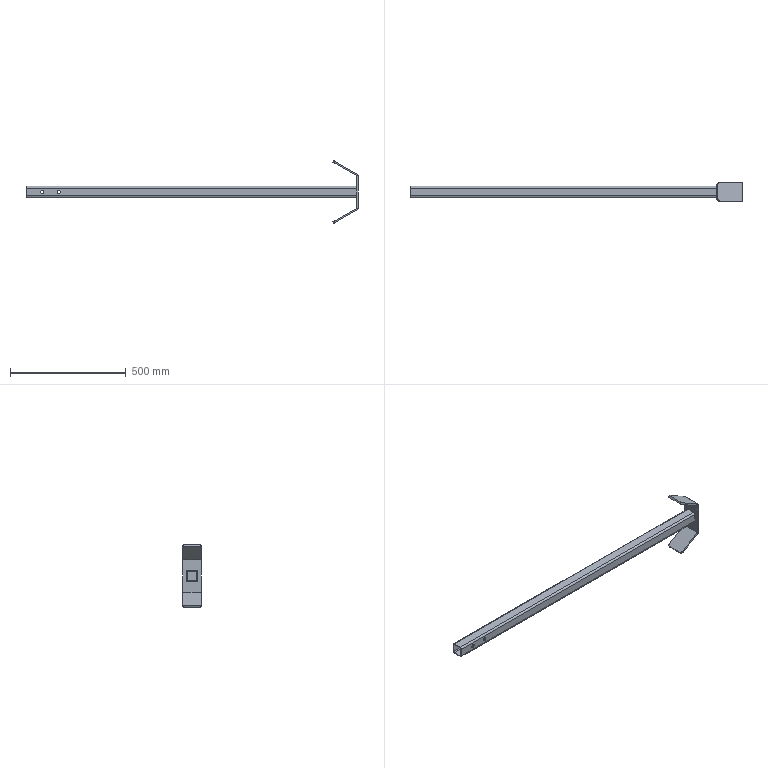Part | SolidWorks | features 3DProfileFeature 1, EdgeFlange 1, Fillet 1, FlatPattern 1, HoleWzd 1, SMBaseFlange 1, SheetMetal 1, WeldMemberFeat 1, WeldmentFeature 1 | 2 solids | 52 faces | box 1433 x 80 x 270.762 mm | volume 1230459 mm3 | plane 28 | cylinder 24 | commonest cylinder face diameters 14 x8 8 x4 16 x4 20 x4 1.473 x2 17.473 x2
STEP:
#1=CARTESIAN_POINT('',(70.,21.,7.));
#2=VERTEX_POINT('',#1);
#3=CARTESIAN_POINT('',(70.,21.,-7.));
#4=VERTEX_POINT('',#3);
#5=CARTESIAN_POINT('',(70.,21.,0.));
#6=DIRECTION('',(0.,-1.,0.));
#7=DIRECTION('',(0.,0.,-1.));
#8=AXIS2_PLACEMENT_3D('',#5,#6,#7);
#9=CIRCLE('',#8,7.);
#10=EDGE_CURVE('',#2,#4,#9,.T.);
#11=ORIENTED_EDGE('',*,*,#10,.T.);
#12=CARTESIAN_POINT('',(70.,25.,-7.));
#13=VERTEX_POINT('',#12);
#14=CARTESIAN_POINT('',(70.,25.,-7.));
#15=DIRECTION('',(0.,1.,0.));
#16=VECTOR('',#15,1000.);
#17=LINE('',#14,#16);
#18=EDGE_CURVE('',#4,#13,#17,.T.);
#19=ORIENTED_EDGE('',*,*,#18,.T.);
#20=CARTESIAN_POINT('',(70.,25.,7.));
#21=VERTEX_POINT('',#20);
#22=CARTESIAN_POINT('',(70.,25.,0.));
#23=DIRECTION('',(0.,1.,0.));
#24=DIRECTION('',(0.,0.,1.));
#25=AXIS2_PLACEMENT_3D('',#22,#23,#24);
#26=CIRCLE('',#25,7.);
#27=EDGE_CURVE('',#13,#21,#26,.T.);
#28=ORIENTED_EDGE('',*,*,#27,.T.);
#29=CARTESIAN_POINT('',(70.,25.,7.));
#30=DIRECTION('',(0.,1.,0.));
#31=VECTOR('',#30,1000.);
#32=LINE('',#29,#31);
#33=EDGE_CURVE('',#2,#21,#32,.T.);
#34=ORIENTED_EDGE('',*,*,#33,.F.);
#35=EDGE_LOOP('',(#11,#19,#28,#34));
#36=FACE_OUTER_BOUND('',#35,.T.);
#37=CARTESIAN_POINT('',(70.,25.,0.));
#38=DIRECTION('',(0.,1.,0.));
#39=DIRECTION('',(0.,0.,1.));
#40=AXIS2_PLACEMENT_3D('',#37,#38,#39);
#41=CYLINDRICAL_SURFACE('',#40,7.);
#42=ADVANCED_FACE('',(#36),#41,.F.);
#43=CARTESIAN_POINT('',(70.,-25.,7.));
#44=VERTEX_POINT('',#43);
#45=CARTESIAN_POINT('',(70.,-25.,-7.));
#46=VERTEX_POINT('',#45);
#47=CARTESIAN_POINT('',(70.,-25.,0.));
#48=DIRECTION('',(0.,-1.,0.));
#49=DIRECTION('',(0.,0.,1.));
#50=AXIS2_PLACEMENT_3D('',#47,#48,#49);
#51=CIRCLE('',#50,7.);
#52=EDGE_CURVE('',#44,#46,#51,.T.);
#53=ORIENTED_EDGE('',*,*,#52,.T.);
#54=CARTESIAN_POINT('',(70.,-21.,-7.));
#55=VERTEX_POINT('',#54);
#56=CARTESIAN_POINT('',(70.,25.,-7.));
#57=DIRECTION('',(0.,1.,0.));
#58=VECTOR('',#57,1000.);
#59=LINE('',#56,#58);
#60=EDGE_CURVE('',#46,#55,#59,.T.);
#61=ORIENTED_EDGE('',*,*,#60,.T.);
#62=CARTESIAN_POINT('',(70.,-21.,7.));
#63=VERTEX_POINT('',#62);
#64=CARTESIAN_POINT('',(70.,-21.,0.));
#65=DIRECTION('',(0.,1.,0.));
#66=DIRECTION('',(0.,0.,1.));
#67=AXIS2_PLACEMENT_3D('',#64,#65,#66);
#68=CIRCLE('',#67,7.);
#69=EDGE_CURVE('',#55,#63,#68,.T.);
#70=ORIENTED_EDGE('',*,*,#69,.T.);
#71=CARTESIAN_POINT('',(70.,25.,7.));
#72=DIRECTION('',(0.,1.,0.));
#73=VECTOR('',#72,1000.);
#74=LINE('',#71,#73);
#75=EDGE_CURVE('',#44,#63,#74,.T.);
#76=ORIENTED_EDGE('',*,*,#75,.F.);
#77=EDGE_LOOP('',(#53,#61,#70,#76));
#78=FACE_OUTER_BOUND('',#77,.T.);
#79=CARTESIAN_POINT('',(70.,25.,0.));
#80=DIRECTION('',(0.,1.,0.));
#81=DIRECTION('',(0.,0.,1.));
#82=AXIS2_PLACEMENT_3D('',#79,#80,#81);
#83=CYLINDRICAL_SURFACE('',#82,7.);
#84=ADVANCED_FACE('',(#78),#83,.F.);
#85=CARTESIAN_POINT('',(141.,21.,7.));
#86=VERTEX_POINT('',#85);
#87=CARTESIAN_POINT('',(141.,21.,-7.));
#88=VERTEX_POINT('',#87);
#89=CARTESIAN_POINT('',(141.,21.,0.));
#90=DIRECTION('',(0.,-1.,0.));
#91=DIRECTION('',(0.,0.,-1.));
#92=AXIS2_PLACEMENT_3D('',#89,#90,#91);
#93=CIRCLE('',#92,7.);
#94=EDGE_CURVE('',#86,#88,#93,.T.);
#95=ORIENTED_EDGE('',*,*,#94,.T.);
#96=CARTESIAN_POINT('',(141.,25.,-7.));
#97=VERTEX_POINT('',#96);
#98=CARTESIAN_POINT('',(141.,25.,-7.));
#99=DIRECTION('',(0.,1.,0.));
#100=VECTOR('',#99,1000.);
#101=LINE('',#98,#100);
#102=EDGE_CURVE('',#88,#97,#101,.T.);
#103=ORIENTED_EDGE('',*,*,#102,.T.);
#104=CARTESIAN_POINT('',(141.,25.,7.));
#105=VERTEX_POINT('',#104);
#106=CARTESIAN_POINT('',(141.,25.,0.));
#107=DIRECTION('',(0.,1.,0.));
#108=DIRECTION('',(0.,0.,1.));
#109=AXIS2_PLACEMENT_3D('',#106,#107,#108);
#110=CIRCLE('',#109,7.);
#111=EDGE_CURVE('',#97,#105,#110,.T.);
#112=ORIENTED_EDGE('',*,*,#111,.T.);
#113=CARTESIAN_POINT('',(141.,25.,7.));
#114=DIRECTION('',(0.,1.,0.));
#115=VECTOR('',#114,1000.);
#116=LINE('',#113,#115);
#117=EDGE_CURVE('',#86,#105,#116,.T.);
#118=ORIENTED_EDGE('',*,*,#117,.F.);
#119=EDGE_LOOP('',(#95,#103,#112,#118));
#120=FACE_OUTER_BOUND('',#119,.T.);
#121=CARTESIAN_POINT('',(141.,25.,0.));
#122=DIRECTION('',(0.,1.,0.));
#123=DIRECTION('',(0.,0.,1.));
#124=AXIS2_PLACEMENT_3D('',#121,#122,#123);
#125=CYLINDRICAL_SURFACE('',#124,7.);
#126=ADVANCED_FACE('',(#120),#125,.F.);
#127=CARTESIAN_POINT('',(141.,-25.,7.));
#128=VERTEX_POINT('',#127);
#129=CARTESIAN_POINT('',(141.,-25.,-7.));
#130=VERTEX_POINT('',#129);
#131=CARTESIAN_POINT('',(141.,-25.,0.));
#132=DIRECTION('',(0.,-1.,0.));
#133=DIRECTION('',(0.,0.,1.));
#134=AXIS2_PLACEMENT_3D('',#131,#132,#133);
#135=CIRCLE('',#134,7.);
#136=EDGE_CURVE('',#128,#130,#135,.T.);
#137=ORIENTED_EDGE('',*,*,#136,.T.);
#138=CARTESIAN_POINT('',(141.,-21.,-7.));
#139=VERTEX_POINT('',#138);
#140=CARTESIAN_POINT('',(141.,25.,-7.));
#141=DIRECTION('',(0.,1.,0.));
#142=VECTOR('',#141,1000.);
#143=LINE('',#140,#142);
#144=EDGE_CURVE('',#130,#139,#143,.T.);
#145=ORIENTED_EDGE('',*,*,#144,.T.);
#146=CARTESIAN_POINT('',(141.,-21.,7.));
#147=VERTEX_POINT('',#146);
#148=CARTESIAN_POINT('',(141.,-21.,0.));
#149=DIRECTION('',(0.,1.,0.));
#150=DIRECTION('',(0.,0.,1.));
#151=AXIS2_PLACEMENT_3D('',#148,#149,#150);
#152=CIRCLE('',#151,7.);
#153=EDGE_CURVE('',#139,#147,#152,.T.);
#154=ORIENTED_EDGE('',*,*,#153,.T.);
#155=CARTESIAN_POINT('',(141.,25.,7.));
#156=DIRECTION('',(0.,1.,0.));
#157=VECTOR('',#156,1000.);
#158=LINE('',#155,#157);
#159=EDGE_CURVE('',#128,#147,#158,.T.);
#160=ORIENTED_EDGE('',*,*,#159,.F.);
#161=EDGE_LOOP('',(#137,#145,#154,#160));
#162=FACE_OUTER_BOUND('',#161,.T.);
#163=CARTESIAN_POINT('',(141.,25.,0.));
#164=DIRECTION('',(0.,1.,0.));
#165=DIRECTION('',(0.,0.,1.));
#166=AXIS2_PLACEMENT_3D('',#163,#164,#165);
#167=CYLINDRICAL_SURFACE('',#166,7.);
#168=ADVANCED_FACE('',(#162),#167,.F.);
#169=CARTESIAN_POINT('',(0.,17.,-25.));
#170=VERTEX_POINT('',#169);
#171=CARTESIAN_POINT('',(0.,25.,-17.));
#172=VERTEX_POINT('',#171);
#173=CARTESIAN_POINT('',(0.,17.,-17.));
#174=DIRECTION('',(1.,0.,0.));
#175=DIRECTION('',(0.,0.,-1.));
#176=AXIS2_PLACEMENT_3D('',#173,#174,#175);
#177=CIRCLE('',#176,8.);
#178=EDGE_CURVE('',#170,#172,#177,.T.);
#179=ORIENTED_EDGE('',*,*,#178,.T.);
#180=CARTESIAN_POINT('',(1425.,25.,-17.));
#181=VERTEX_POINT('',#180);
#182=CARTESIAN_POINT('',(1425.,25.,-17.));
#183=DIRECTION('',(-1.,0.,0.));
#184=VECTOR('',#183,1000.);
#185=LINE('',#182,#184);
#186=EDGE_CURVE('',#181,#172,#185,.T.);
#187=ORIENTED_EDGE('',*,*,#186,.F.);
#188=CARTESIAN_POINT('',(1425.,17.,-25.));
#189=VERTEX_POINT('',#188);
#190=CARTESIAN_POINT('',(1425.,17.,-17.));
#191=DIRECTION('',(1.,0.,0.));
#192=DIRECTION('',(0.,0.,-1.));
#193=AXIS2_PLACEMENT_3D('',#190,#191,#192);
#194=CIRCLE('',#193,8.);
#195=EDGE_CURVE('',#189,#181,#194,.T.);
#196=ORIENTED_EDGE('',*,*,#195,.F.);
#197=CARTESIAN_POINT('',(1425.,17.,-25.));
#198=DIRECTION('',(-1.,0.,0.));
#199=VECTOR('',#198,1000.);
#200=LINE('',#197,#199);
#201=EDGE_CURVE('',#189,#170,#200,.T.);
#202=ORIENTED_EDGE('',*,*,#201,.T.);
#203=EDGE_LOOP('',(#179,#187,#196,#202));
#204=FACE_OUTER_BOUND('',#203,.T.);
#205=CARTESIAN_POINT('',(1425.,17.,-17.));
#206=DIRECTION('',(-1.,0.,0.));
#207=DIRECTION('',(0.,0.,1.));
#208=AXIS2_PLACEMENT_3D('',#205,#206,#207);
#209=CYLINDRICAL_SURFACE('',#208,8.);
#210=ADVANCED_FACE('',(#204),#209,.T.);
#211=CARTESIAN_POINT('',(70.,25.,0.));
#212=DIRECTION('',(0.,1.,0.));
#213=DIRECTION('',(0.,0.,1.));
#214=AXIS2_PLACEMENT_3D('',#211,#212,#213);
#215=CIRCLE('',#214,7.);
#216=EDGE_CURVE('',#21,#13,#215,.T.);
#217=ORIENTED_EDGE('',*,*,#216,.F.);
#218=ORIENTED_EDGE('',*,*,#27,.F.);
#219=EDGE_LOOP('',(#217,#218));
#220=FACE_BOUND('',#219,.T.);
#221=CARTESIAN_POINT('',(141.,25.,0.));
#222=DIRECTION('',(0.,1.,0.));
#223=DIRECTION('',(0.,0.,1.));
#224=AXIS2_PLACEMENT_3D('',#221,#222,#223);
#225=CIRCLE('',#224,7.);
#226=EDGE_CURVE('',#105,#97,#225,.T.);
#227=ORIENTED_EDGE('',*,*,#226,.F.);
#228=ORIENTED_EDGE('',*,*,#111,.F.);
#229=EDGE_LOOP('',(#227,#228));
#230=FACE_BOUND('',#229,.T.);
#231=CARTESIAN_POINT('',(0.,25.,17.));
#232=VERTEX_POINT('',#231);
#233=CARTESIAN_POINT('',(0.,25.,-17.));
#234=DIRECTION('',(0.,0.,1.));
#235=VECTOR('',#234,1000.);
#236=LINE('',#233,#235);
#237=EDGE_CURVE('',#172,#232,#236,.T.);
#238=ORIENTED_EDGE('',*,*,#237,.T.);
#239=CARTESIAN_POINT('',(1425.,25.,17.));
#240=VERTEX_POINT('',#239);
#241=CARTESIAN_POINT('',(1425.,25.,17.));
#242=DIRECTION('',(-1.,0.,0.));
#243=VECTOR('',#242,1000.);
#244=LINE('',#241,#243);
#245=EDGE_CURVE('',#240,#232,#244,.T.);
#246=ORIENTED_EDGE('',*,*,#245,.F.);
#247=CARTESIAN_POINT('',(1425.,25.,-17.));
#248=DIRECTION('',(0.,0.,1.));
#249=VECTOR('',#248,1000.);
#250=LINE('',#247,#249);
#251=EDGE_CURVE('',#181,#240,#250,.T.);
#252=ORIENTED_EDGE('',*,*,#251,.F.);
#253=ORIENTED_EDGE('',*,*,#186,.T.);
#254=EDGE_LOOP('',(#238,#246,#252,#253));
#255=FACE_OUTER_BOUND('',#254,.T.);
#256=CARTESIAN_POINT('',(1425.,25.,-17.));
#257=DIRECTION('',(0.,-1.,0.));
#258=DIRECTION('',(0.,0.,-1.));
#259=AXIS2_PLACEMENT_3D('',#256,#257,#258);
#260=PLANE('',#259);
#261=ADVANCED_FACE('',(#220,#230,#255),#260,.F.);
#262=CARTESIAN_POINT('',(0.,17.,25.));
#263=VERTEX_POINT('',#262);
#264=CARTESIAN_POINT('',(0.,17.,17.));
#265=DIRECTION('',(1.,0.,0.));
#266=DIRECTION('',(0.,0.,-1.));
#267=AXIS2_PLACEMENT_3D('',#264,#265,#266);
#268=CIRCLE('',#267,8.);
#269=EDGE_CURVE('',#232,#263,#268,.T.);
#270=ORIENTED_EDGE('',*,*,#269,.T.);
#271=CARTESIAN_POINT('',(1425.,17.,25.));
#272=VERTEX_POINT('',#271);
#273=CARTESIAN_POINT('',(1425.,17.,25.));
#274=DIRECTION('',(-1.,0.,0.));
#275=VECTOR('',#274,1000.);
#276=LINE('',#273,#275);
#277=EDGE_CURVE('',#272,#263,#276,.T.);
#278=ORIENTED_EDGE('',*,*,#277,.F.);
#279=CARTESIAN_POINT('',(1425.,17.,17.));
#280=DIRECTION('',(1.,0.,0.));
#281=DIRECTION('',(0.,0.,-1.));
#282=AXIS2_PLACEMENT_3D('',#279,#280,#281);
#283=CIRCLE('',#282,8.);
#284=EDGE_CURVE('',#240,#272,#283,.T.);
#285=ORIENTED_EDGE('',*,*,#284,.F.);
#286=ORIENTED_EDGE('',*,*,#245,.T.);
#287=EDGE_LOOP('',(#270,#278,#285,#286));
#288=FACE_OUTER_BOUND('',#287,.T.);
#289=CARTESIAN_POINT('',(1425.,17.,17.));
#290=DIRECTION('',(-1.,0.,0.));
#291=DIRECTION('',(0.,0.,1.));
#292=AXIS2_PLACEMENT_3D('',#289,#290,#291);
#293=CYLINDRICAL_SURFACE('',#292,8.);
#294=ADVANCED_FACE('',(#288),#293,.T.);
#295=CARTESIAN_POINT('',(0.,-17.,25.));
#296=VERTEX_POINT('',#295);
#297=CARTESIAN_POINT('',(0.,-17.,25.));
#298=DIRECTION('',(0.,-1.,0.));
#299=VECTOR('',#298,1000.);
#300=LINE('',#297,#299);
#301=EDGE_CURVE('',#263,#296,#300,.T.);
#302=ORIENTED_EDGE('',*,*,#301,.T.);
#303=CARTESIAN_POINT('',(1425.,-17.,25.));
#304=VERTEX_POINT('',#303);
#305=CARTESIAN_POINT('',(1425.,-17.,25.));
#306=DIRECTION('',(-1.,0.,0.));
#307=VECTOR('',#306,1000.);
#308=LINE('',#305,#307);
#309=EDGE_CURVE('',#304,#296,#308,.T.);
#310=ORIENTED_EDGE('',*,*,#309,.F.);
#311=CARTESIAN_POINT('',(1425.,-17.,25.));
#312=DIRECTION('',(0.,-1.,0.));
#313=VECTOR('',#312,1000.);
#314=LINE('',#311,#313);
#315=EDGE_CURVE('',#272,#304,#314,.T.);
#316=ORIENTED_EDGE('',*,*,#315,.F.);
#317=ORIENTED_EDGE('',*,*,#277,.T.);
#318=EDGE_LOOP('',(#302,#310,#316,#317));
#319=FACE_OUTER_BOUND('',#318,.T.);
#320=CARTESIAN_POINT('',(1425.,-17.,25.));
#321=DIRECTION('',(0.,0.,-1.));
#322=DIRECTION('',(-1.,0.,0.));
#323=AXIS2_PLACEMENT_3D('',#320,#321,#322);
#324=PLANE('',#323);
#325=ADVANCED_FACE('',(#319),#324,.F.);
#326=CARTESIAN_POINT('',(0.,-25.,17.));
#327=VERTEX_POINT('',#326);
#328=CARTESIAN_POINT('',(0.,-17.,17.));
#329=DIRECTION('',(1.,0.,0.));
#330=DIRECTION('',(0.,0.,-1.));
#331=AXIS2_PLACEMENT_3D('',#328,#329,#330);
#332=CIRCLE('',#331,8.);
#333=EDGE_CURVE('',#296,#327,#332,.T.);
#334=ORIENTED_EDGE('',*,*,#333,.T.);
#335=CARTESIAN_POINT('',(1425.,-25.,17.));
#336=VERTEX_POINT('',#335);
#337=CARTESIAN_POINT('',(1425.,-25.,17.));
#338=DIRECTION('',(-1.,0.,0.));
#339=VECTOR('',#338,1000.);
#340=LINE('',#337,#339);
#341=EDGE_CURVE('',#336,#327,#340,.T.);
#342=ORIENTED_EDGE('',*,*,#341,.F.);
#343=CARTESIAN_POINT('',(1425.,-17.,17.));
#344=DIRECTION('',(1.,0.,0.));
#345=DIRECTION('',(0.,0.,-1.));
#346=AXIS2_PLACEMENT_3D('',#343,#344,#345);
#347=CIRCLE('',#346,8.);
#348=EDGE_CURVE('',#304,#336,#347,.T.);
#349=ORIENTED_EDGE('',*,*,#348,.F.);
#350=ORIENTED_EDGE('',*,*,#309,.T.);
#351=EDGE_LOOP('',(#334,#342,#349,#350));
#352=FACE_OUTER_BOUND('',#351,.T.);
#353=CARTESIAN_POINT('',(1425.,-17.,17.));
#354=DIRECTION('',(-1.,0.,0.));
#355=DIRECTION('',(0.,0.,1.));
#356=AXIS2_PLACEMENT_3D('',#353,#354,#355);
#357=CYLINDRICAL_SURFACE('',#356,8.);
#358=ADVANCED_FACE('',(#352),#357,.T.);
#359=ORIENTED_EDGE('',*,*,#52,.F.);
#360=CARTESIAN_POINT('',(70.,-25.,0.));
#361=DIRECTION('',(0.,-1.,0.));
#362=DIRECTION('',(0.,0.,1.));
#363=AXIS2_PLACEMENT_3D('',#360,#361,#362);
#364=CIRCLE('',#363,7.);
#365=EDGE_CURVE('',#46,#44,#364,.T.);
#366=ORIENTED_EDGE('',*,*,#365,.F.);
#367=EDGE_LOOP('',(#359,#366));
#368=FACE_BOUND('',#367,.T.);
#369=ORIENTED_EDGE('',*,*,#136,.F.);
#370=CARTESIAN_POINT('',(141.,-25.,0.));
#371=DIRECTION('',(0.,-1.,0.));
#372=DIRECTION('',(0.,0.,1.));
#373=AXIS2_PLACEMENT_3D('',#370,#371,#372);
#374=CIRCLE('',#373,7.);
#375=EDGE_CURVE('',#130,#128,#374,.T.);
#376=ORIENTED_EDGE('',*,*,#375,.F.);
#377=EDGE_LOOP('',(#369,#376));
#378=FACE_BOUND('',#377,.T.);
#379=CARTESIAN_POINT('',(0.,-25.,-17.));
#380=VERTEX_POINT('',#379);
#381=CARTESIAN_POINT('',(0.,-25.,17.));
#382=DIRECTION('',(0.,0.,-1.));
#383=VECTOR('',#382,1000.);
#384=LINE('',#381,#383);
#385=EDGE_CURVE('',#327,#380,#384,.T.);
#386=ORIENTED_EDGE('',*,*,#385,.T.);
#387=CARTESIAN_POINT('',(1425.,-25.,-17.));
#388=VERTEX_POINT('',#387);
#389=CARTESIAN_POINT('',(1425.,-25.,-17.));
#390=DIRECTION('',(-1.,0.,0.));
#391=VECTOR('',#390,1000.);
#392=LINE('',#389,#391);
#393=EDGE_CURVE('',#388,#380,#392,.T.);
#394=ORIENTED_EDGE('',*,*,#393,.F.);
#395=CARTESIAN_POINT('',(1425.,-25.,17.));
#396=DIRECTION('',(0.,0.,-1.));
#397=VECTOR('',#396,1000.);
#398=LINE('',#395,#397);
#399=EDGE_CURVE('',#336,#388,#398,.T.);
#400=ORIENTED_EDGE('',*,*,#399,.F.);
#401=ORIENTED_EDGE('',*,*,#341,.T.);
#402=EDGE_LOOP('',(#386,#394,#400,#401));
#403=FACE_OUTER_BOUND('',#402,.T.);
#404=CARTESIAN_POINT('',(1425.,-25.,17.));
#405=DIRECTION('',(0.,1.,0.));
#406=DIRECTION('',(0.,0.,1.));
#407=AXIS2_PLACEMENT_3D('',#404,#405,#406);
#408=PLANE('',#407);
#409=ADVANCED_FACE('',(#368,#378,#403),#408,.F.);
#410=CARTESIAN_POINT('',(0.,-17.,-25.));
#411=VERTEX_POINT('',#410);
#412=CARTESIAN_POINT('',(0.,-17.,-17.));
#413=DIRECTION('',(1.,0.,0.));
#414=DIRECTION('',(0.,0.,-1.));
#415=AXIS2_PLACEMENT_3D('',#412,#413,#414);
#416=CIRCLE('',#415,8.);
#417=EDGE_CURVE('',#380,#411,#416,.T.);
#418=ORIENTED_EDGE('',*,*,#417,.T.);
#419=CARTESIAN_POINT('',(1425.,-17.,-25.));
#420=VERTEX_POINT('',#419);
#421=CARTESIAN_POINT('',(1425.,-17.,-25.));
#422=DIRECTION('',(-1.,0.,0.));
#423=VECTOR('',#422,1000.);
#424=LINE('',#421,#423);
#425=EDGE_CURVE('',#420,#411,#424,.T.);
#426=ORIENTED_EDGE('',*,*,#425,.F.);
#427=CARTESIAN_POINT('',(1425.,-17.,-17.));
#428=DIRECTION('',(1.,0.,0.));
#429=DIRECTION('',(0.,0.,-1.));
#430=AXIS2_PLACEMENT_3D('',#427,#428,#429);
#431=CIRCLE('',#430,8.);
#432=EDGE_CURVE('',#388,#420,#431,.T.);
#433=ORIENTED_EDGE('',*,*,#432,.F.);
#434=ORIENTED_EDGE('',*,*,#393,.T.);
#435=EDGE_LOOP('',(#418,#426,#433,#434));
#436=FACE_OUTER_BOUND('',#435,.T.);
#437=CARTESIAN_POINT('',(1425.,-17.,-17.));
#438=DIRECTION('',(-1.,0.,0.));
#439=DIRECTION('',(0.,0.,1.));
#440=AXIS2_PLACEMENT_3D('',#437,#438,#439);
#441=CYLINDRICAL_SURFACE('',#440,8.);
#442=ADVANCED_FACE('',(#436),#441,.T.);
#443=CARTESIAN_POINT('',(0.,21.,17.));
#444=VERTEX_POINT('',#443);
#445=CARTESIAN_POINT('',(0.,17.,21.));
#446=VERTEX_POINT('',#445);
#447=CARTESIAN_POINT('',(0.,17.,17.));
#448=DIRECTION('',(1.,0.,0.));
#449=DIRECTION('',(0.,0.,-1.));
#450=AXIS2_PLACEMENT_3D('',#447,#448,#449);
#451=CIRCLE('',#450,4.);
#452=EDGE_CURVE('',#444,#446,#451,.T.);
#453=ORIENTED_EDGE('',*,*,#452,.F.);
#454=CARTESIAN_POINT('',(1425.,21.,17.));
#455=VERTEX_POINT('',#454);
#456=CARTESIAN_POINT('',(1425.,21.,17.));
#457=DIRECTION('',(-1.,0.,0.));
#458=VECTOR('',#457,1000.);
#459=LINE('',#456,#458);
#460=EDGE_CURVE('',#455,#444,#459,.T.);
#461=ORIENTED_EDGE('',*,*,#460,.F.);
#462=CARTESIAN_POINT('',(1425.,17.,21.));
#463=VERTEX_POINT('',#462);
#464=CARTESIAN_POINT('',(1425.,17.,17.));
#465=DIRECTION('',(1.,0.,0.));
#466=DIRECTION('',(0.,0.,-1.));
#467=AXIS2_PLACEMENT_3D('',#464,#465,#466);
#468=CIRCLE('',#467,4.);
#469=EDGE_CURVE('',#455,#463,#468,.T.);
#470=ORIENTED_EDGE('',*,*,#469,.T.);
#471=CARTESIAN_POINT('',(1425.,17.,21.));
#472=DIRECTION('',(-1.,0.,0.));
#473=VECTOR('',#472,1000.);
#474=LINE('',#471,#473);
#475=EDGE_CURVE('',#463,#446,#474,.T.);
#476=ORIENTED_EDGE('',*,*,#475,.T.);
#477=EDGE_LOOP('',(#453,#461,#470,#476));
#478=FACE_OUTER_BOUND('',#477,.T.);
#479=CARTESIAN_POINT('',(1425.,17.,17.));
#480=DIRECTION('',(-1.,0.,0.));
#481=DIRECTION('',(0.,0.,1.));
#482=AXIS2_PLACEMENT_3D('',#479,#480,#481);
#483=CYLINDRICAL_SURFACE('',#482,4.);
#484=ADVANCED_FACE('',(#478),#483,.F.);
#485=ORIENTED_EDGE('',*,*,#10,.F.);
#486=CARTESIAN_POINT('',(70.,21.,0.));
#487=DIRECTION('',(0.,-1.,0.));
#488=DIRECTION('',(0.,0.,-1.));
#489=AXIS2_PLACEMENT_3D('',#486,#487,#488);
#490=CIRCLE('',#489,7.);
#491=EDGE_CURVE('',#4,#2,#490,.T.);
#492=ORIENTED_EDGE('',*,*,#491,.F.);
#493=EDGE_LOOP('',(#485,#492));
#494=FACE_BOUND('',#493,.T.);
#495=ORIENTED_EDGE('',*,*,#94,.F.);
#496=CARTESIAN_POINT('',(141.,21.,0.));
#497=DIRECTION('',(0.,-1.,0.));
#498=DIRECTION('',(0.,0.,-1.));
#499=AXIS2_PLACEMENT_3D('',#496,#497,#498);
#500=CIRCLE('',#499,7.);
#501=EDGE_CURVE('',#88,#86,#500,.T.);
#502=ORIENTED_EDGE('',*,*,#501,.F.);
#503=EDGE_LOOP('',(#495,#502));
#504=FACE_BOUND('',#503,.T.);
#505=CARTESIAN_POINT('',(0.,21.,-17.));
#506=VERTEX_POINT('',#505);
#507=CARTESIAN_POINT('',(0.,21.,-17.));
#508=DIRECTION('',(0.,0.,1.));
#509=VECTOR('',#508,1000.);
#510=LINE('',#507,#509);
#511=EDGE_CURVE('',#506,#444,#510,.T.);
#512=ORIENTED_EDGE('',*,*,#511,.F.);
#513=CARTESIAN_POINT('',(1425.,21.,-17.));
#514=VERTEX_POINT('',#513);
#515=CARTESIAN_POINT('',(1425.,21.,-17.));
#516=DIRECTION('',(-1.,0.,0.));
#517=VECTOR('',#516,1000.);
#518=LINE('',#515,#517);
#519=EDGE_CURVE('',#514,#506,#518,.T.);
#520=ORIENTED_EDGE('',*,*,#519,.F.);
#521=CARTESIAN_POINT('',(1425.,21.,-17.));
#522=DIRECTION('',(0.,0.,1.));
#523=VECTOR('',#522,1000.);
#524=LINE('',#521,#523);
#525=EDGE_CURVE('',#514,#455,#524,.T.);
#526=ORIENTED_EDGE('',*,*,#525,.T.);
#527=ORIENTED_EDGE('',*,*,#460,.T.);
#528=EDGE_LOOP('',(#512,#520,#526,#527));
#529=FACE_OUTER_BOUND('',#528,.T.);
#530=CARTESIAN_POINT('',(1425.,21.,-17.));
#531=DIRECTION('',(0.,-1.,0.));
#532=DIRECTION('',(0.,0.,-1.));
#533=AXIS2_PLACEMENT_3D('',#530,#531,#532);
#534=PLANE('',#533);
#535=ADVANCED_FACE('',(#494,#504,#529),#534,.T.);
#536=CARTESIAN_POINT('',(0.,17.,-21.));
#537=VERTEX_POINT('',#536);
#538=CARTESIAN_POINT('',(0.,17.,-17.));
#539=DIRECTION('',(1.,0.,0.));
#540=DIRECTION('',(0.,0.,-1.));
#541=AXIS2_PLACEMENT_3D('',#538,#539,#540);
#542=CIRCLE('',#541,4.);
#543=EDGE_CURVE('',#537,#506,#542,.T.);
#544=ORIENTED_EDGE('',*,*,#543,.F.);
#545=CARTESIAN_POINT('',(1425.,17.,-21.));
#546=VERTEX_POINT('',#545);
#547=CARTESIAN_POINT('',(1425.,17.,-21.));
#548=DIRECTION('',(-1.,0.,0.));
#549=VECTOR('',#548,1000.);
#550=LINE('',#547,#549);
#551=EDGE_CURVE('',#546,#537,#550,.T.);
#552=ORIENTED_EDGE('',*,*,#551,.F.);
#553=CARTESIAN_POINT('',(1425.,17.,-17.));
#554=DIRECTION('',(1.,0.,0.));
#555=DIRECTION('',(0.,0.,-1.));
#556=AXIS2_PLACEMENT_3D('',#553,#554,#555);
#557=CIRCLE('',#556,4.);
#558=EDGE_CURVE('',#546,#514,#557,.T.);
#559=ORIENTED_EDGE('',*,*,#558,.T.);
#560=ORIENTED_EDGE('',*,*,#519,.T.);
#561=EDGE_LOOP('',(#544,#552,#559,#560));
#562=FACE_OUTER_BOUND('',#561,.T.);
#563=CARTESIAN_POINT('',(1425.,17.,-17.));
#564=DIRECTION('',(-1.,0.,0.));
#565=DIRECTION('',(0.,0.,1.));
#566=AXIS2_PLACEMENT_3D('',#563,#564,#565);
#567=CYLINDRICAL_SURFACE('',#566,4.);
#568=ADVANCED_FACE('',(#562),#567,.F.);
#569=CARTESIAN_POINT('',(0.,-17.,-21.));
#570=VERTEX_POINT('',#569);
#571=CARTESIAN_POINT('',(0.,17.,-21.));
#572=DIRECTION('',(0.,1.,0.));
#573=VECTOR('',#572,1000.);
#574=LINE('',#571,#573);
#575=EDGE_CURVE('',#570,#537,#574,.T.);
#576=ORIENTED_EDGE('',*,*,#575,.F.);
#577=CARTESIAN_POINT('',(1425.,-17.,-21.));
#578=VERTEX_POINT('',#577);
#579=CARTESIAN_POINT('',(1425.,-17.,-21.));
#580=DIRECTION('',(-1.,0.,0.));
#581=VECTOR('',#580,1000.);
#582=LINE('',#579,#581);
#583=EDGE_CURVE('',#578,#570,#582,.T.);
#584=ORIENTED_EDGE('',*,*,#583,.F.);
#585=CARTESIAN_POINT('',(1425.,17.,-21.));
#586=DIRECTION('',(0.,1.,0.));
#587=VECTOR('',#586,1000.);
#588=LINE('',#585,#587);
#589=EDGE_CURVE('',#578,#546,#588,.T.);
#590=ORIENTED_EDGE('',*,*,#589,.T.);
#591=ORIENTED_EDGE('',*,*,#551,.T.);
#592=EDGE_LOOP('',(#576,#584,#590,#591));
#593=FACE_OUTER_BOUND('',#592,.T.);
#594=CARTESIAN_POINT('',(1425.,17.,-21.));
#595=DIRECTION('',(0.,0.,1.));
#596=DIRECTION('',(1.,0.,0.));
#597=AXIS2_PLACEMENT_3D('',#594,#595,#596);
#598=PLANE('',#597);
#599=ADVANCED_FACE('',(#593),#598,.T.);
#600=CARTESIAN_POINT('',(0.,-21.,-17.));
#601=VERTEX_POINT('',#600);
#602=CARTESIAN_POINT('',(0.,-17.,-17.));
#603=DIRECTION('',(1.,0.,0.));
#604=DIRECTION('',(0.,0.,-1.));
#605=AXIS2_PLACEMENT_3D('',#602,#603,#604);
#606=CIRCLE('',#605,4.);
#607=EDGE_CURVE('',#601,#570,#606,.T.);
#608=ORIENTED_EDGE('',*,*,#607,.F.);
#609=CARTESIAN_POINT('',(1425.,-21.,-17.));
#610=VERTEX_POINT('',#609);
#611=CARTESIAN_POINT('',(1425.,-21.,-17.));
#612=DIRECTION('',(-1.,0.,0.));
#613=VECTOR('',#612,1000.);
#614=LINE('',#611,#613);
#615=EDGE_CURVE('',#610,#601,#614,.T.);
#616=ORIENTED_EDGE('',*,*,#615,.F.);
#617=CARTESIAN_POINT('',(1425.,-17.,-17.));
#618=DIRECTION('',(1.,0.,0.));
#619=DIRECTION('',(0.,0.,-1.));
#620=AXIS2_PLACEMENT_3D('',#617,#618,#619);
#621=CIRCLE('',#620,4.);
#622=EDGE_CURVE('',#610,#578,#621,.T.);
#623=ORIENTED_EDGE('',*,*,#622,.T.);
#624=ORIENTED_EDGE('',*,*,#583,.T.);
#625=EDGE_LOOP('',(#608,#616,#623,#624));
#626=FACE_OUTER_BOUND('',#625,.T.);
#627=CARTESIAN_POINT('',(1425.,-17.,-17.));
#628=DIRECTION('',(-1.,0.,0.));
#629=DIRECTION('',(0.,0.,1.));
#630=AXIS2_PLACEMENT_3D('',#627,#628,#629);
#631=CYLINDRICAL_SURFACE('',#630,4.);
#632=ADVANCED_FACE('',(#626),#631,.F.);
#633=CARTESIAN_POINT('',(70.,-21.,0.));
#634=DIRECTION('',(0.,1.,0.));
#635=DIRECTION('',(0.,0.,1.));
#636=AXIS2_PLACEMENT_3D('',#633,#634,#635);
#637=CIRCLE('',#636,7.);
#638=EDGE_CURVE('',#63,#55,#637,.T.);
#639=ORIENTED_EDGE('',*,*,#638,.F.);
#640=ORIENTED_EDGE('',*,*,#69,.F.);
#641=EDGE_LOOP('',(#639,#640));
#642=FACE_BOUND('',#641,.T.);
#643=CARTESIAN_POINT('',(141.,-21.,0.));
#644=DIRECTION('',(0.,1.,0.));
#645=DIRECTION('',(0.,0.,1.));
#646=AXIS2_PLACEMENT_3D('',#643,#644,#645);
#647=CIRCLE('',#646,7.);
#648=EDGE_CURVE('',#147,#139,#647,.T.);
#649=ORIENTED_EDGE('',*,*,#648,.F.);
#650=ORIENTED_EDGE('',*,*,#153,.F.);
#651=EDGE_LOOP('',(#649,#650));
#652=FACE_BOUND('',#651,.T.);
#653=CARTESIAN_POINT('',(0.,-21.,17.));
#654=VERTEX_POINT('',#653);
#655=CARTESIAN_POINT('',(0.,-21.,17.));
#656=DIRECTION('',(0.,0.,-1.));
#657=VECTOR('',#656,1000.);
#658=LINE('',#655,#657);
#659=EDGE_CURVE('',#654,#601,#658,.T.);
#660=ORIENTED_EDGE('',*,*,#659,.F.);
#661=CARTESIAN_POINT('',(1425.,-21.,17.));
#662=VERTEX_POINT('',#661);
#663=CARTESIAN_POINT('',(1425.,-21.,17.));
#664=DIRECTION('',(-1.,0.,0.));
#665=VECTOR('',#664,1000.);
#666=LINE('',#663,#665);
#667=EDGE_CURVE('',#662,#654,#666,.T.);
#668=ORIENTED_EDGE('',*,*,#667,.F.);
#669=CARTESIAN_POINT('',(1425.,-21.,17.));
#670=DIRECTION('',(0.,0.,-1.));
#671=VECTOR('',#670,1000.);
#672=LINE('',#669,#671);
#673=EDGE_CURVE('',#662,#610,#672,.T.);
#674=ORIENTED_EDGE('',*,*,#673,.T.);
#675=ORIENTED_EDGE('',*,*,#615,.T.);
#676=EDGE_LOOP('',(#660,#668,#674,#675));
#677=FACE_OUTER_BOUND('',#676,.T.);
#678=CARTESIAN_POINT('',(1425.,-21.,17.));
#679=DIRECTION('',(0.,1.,0.));
#680=DIRECTION('',(0.,0.,1.));
#681=AXIS2_PLACEMENT_3D('',#678,#679,#680);
#682=PLANE('',#681);
#683=ADVANCED_FACE('',(#642,#652,#677),#682,.T.);
#684=CARTESIAN_POINT('',(0.,-17.,21.));
#685=VERTEX_POINT('',#684);
#686=CARTESIAN_POINT('',(0.,-17.,17.));
#687=DIRECTION('',(1.,0.,0.));
#688=DIRECTION('',(0.,0.,-1.));
#689=AXIS2_PLACEMENT_3D('',#686,#687,#688);
#690=CIRCLE('',#689,4.);
#691=EDGE_CURVE('',#685,#654,#690,.T.);
#692=ORIENTED_EDGE('',*,*,#691,.F.);
#693=CARTESIAN_POINT('',(1425.,-17.,21.));
#694=VERTEX_POINT('',#693);
#695=CARTESIAN_POINT('',(1425.,-17.,21.));
#696=DIRECTION('',(-1.,0.,0.));
#697=VECTOR('',#696,1000.);
#698=LINE('',#695,#697);
#699=EDGE_CURVE('',#694,#685,#698,.T.);
#700=ORIENTED_EDGE('',*,*,#699,.F.);
#701=CARTESIAN_POINT('',(1425.,-17.,17.));
#702=DIRECTION('',(1.,0.,0.));
#703=DIRECTION('',(0.,0.,-1.));
#704=AXIS2_PLACEMENT_3D('',#701,#702,#703);
#705=CIRCLE('',#704,4.);
#706=EDGE_CURVE('',#694,#662,#705,.T.);
#707=ORIENTED_EDGE('',*,*,#706,.T.);
#708=ORIENTED_EDGE('',*,*,#667,.T.);
#709=EDGE_LOOP('',(#692,#700,#707,#708));
#710=FACE_OUTER_BOUND('',#709,.T.);
#711=CARTESIAN_POINT('',(1425.,-17.,17.));
#712=DIRECTION('',(-1.,0.,0.));
#713=DIRECTION('',(0.,0.,1.));
#714=AXIS2_PLACEMENT_3D('',#711,#712,#713);
#715=CYLINDRICAL_SURFACE('',#714,4.);
#716=ADVANCED_FACE('',(#710),#715,.F.);
#717=CARTESIAN_POINT('',(0.,-17.,21.));
#718=DIRECTION('',(0.,-1.,0.));
#719=VECTOR('',#718,1000.);
#720=LINE('',#717,#719);
#721=EDGE_CURVE('',#446,#685,#720,.T.);
#722=ORIENTED_EDGE('',*,*,#721,.F.);
#723=ORIENTED_EDGE('',*,*,#475,.F.);
#724=CARTESIAN_POINT('',(1425.,-17.,21.));
#725=DIRECTION('',(0.,-1.,0.));
#726=VECTOR('',#725,1000.);
#727=LINE('',#724,#726);
#728=EDGE_CURVE('',#463,#694,#727,.T.);
#729=ORIENTED_EDGE('',*,*,#728,.T.);
#730=ORIENTED_EDGE('',*,*,#699,.T.);
#731=EDGE_LOOP('',(#722,#723,#729,#730));
#732=FACE_OUTER_BOUND('',#731,.T.);
#733=CARTESIAN_POINT('',(1425.,-17.,21.));
#734=DIRECTION('',(0.,0.,-1.));
#735=DIRECTION('',(-1.,0.,0.));
#736=AXIS2_PLACEMENT_3D('',#733,#734,#735);
#737=PLANE('',#736);
#738=ADVANCED_FACE('',(#732),#737,.T.);
#739=CARTESIAN_POINT('',(0.,17.,-25.));
#740=DIRECTION('',(0.,1.,0.));
#741=VECTOR('',#740,1000.);
#742=LINE('',#739,#741);
#743=EDGE_CURVE('',#411,#170,#742,.T.);
#744=ORIENTED_EDGE('',*,*,#743,.T.);
#745=ORIENTED_EDGE('',*,*,#201,.F.);
#746=CARTESIAN_POINT('',(1425.,17.,-25.));
#747=DIRECTION('',(0.,1.,0.));
#748=VECTOR('',#747,1000.);
#749=LINE('',#746,#748);
#750=EDGE_CURVE('',#420,#189,#749,.T.);
#751=ORIENTED_EDGE('',*,*,#750,.F.);
#752=ORIENTED_EDGE('',*,*,#425,.T.);
#753=EDGE_LOOP('',(#744,#745,#751,#752));
#754=FACE_OUTER_BOUND('',#753,.T.);
#755=CARTESIAN_POINT('',(1425.,17.,-25.));
#756=DIRECTION('',(0.,0.,1.));
#757=DIRECTION('',(1.,0.,0.));
#758=AXIS2_PLACEMENT_3D('',#755,#756,#757);
#759=PLANE('',#758);
#760=ADVANCED_FACE('',(#754),#759,.F.);
#761=ORIENTED_EDGE('',*,*,#469,.F.);
#762=ORIENTED_EDGE('',*,*,#525,.F.);
#763=ORIENTED_EDGE('',*,*,#558,.F.);
#764=ORIENTED_EDGE('',*,*,#589,.F.);
#765=ORIENTED_EDGE('',*,*,#622,.F.);
#766=ORIENTED_EDGE('',*,*,#673,.F.);
#767=ORIENTED_EDGE('',*,*,#706,.F.);
#768=ORIENTED_EDGE('',*,*,#728,.F.);
#769=EDGE_LOOP('',(#761,#762,#763,#764,#765,#766,#767,#768));
#770=FACE_BOUND('',#769,.T.);
#771=ORIENTED_EDGE('',*,*,#195,.T.);
#772=ORIENTED_EDGE('',*,*,#251,.T.);
#773=ORIENTED_EDGE('',*,*,#284,.T.);
#774=ORIENTED_EDGE('',*,*,#315,.T.);
#775=ORIENTED_EDGE('',*,*,#348,.T.);
#776=ORIENTED_EDGE('',*,*,#399,.T.);
#777=ORIENTED_EDGE('',*,*,#432,.T.);
#778=ORIENTED_EDGE('',*,*,#750,.T.);
#779=EDGE_LOOP('',(#771,#772,#773,#774,#775,#776,#777,#778));
#780=FACE_OUTER_BOUND('',#779,.T.);
#781=CARTESIAN_POINT('',(1425.,17.,-17.));
#782=DIRECTION('',(1.,0.,0.));
#783=DIRECTION('',(0.,0.,-1.));
#784=AXIS2_PLACEMENT_3D('',#781,#782,#783);
#785=PLANE('',#784);
#786=ADVANCED_FACE('',(#770,#780),#785,.T.);
#787=ORIENTED_EDGE('',*,*,#452,.T.);
#788=ORIENTED_EDGE('',*,*,#721,.T.);
#789=ORIENTED_EDGE('',*,*,#691,.T.);
#790=ORIENTED_EDGE('',*,*,#659,.T.);
#791=ORIENTED_EDGE('',*,*,#607,.T.);
#792=ORIENTED_EDGE('',*,*,#575,.T.);
#793=ORIENTED_EDGE('',*,*,#543,.T.);
#794=ORIENTED_EDGE('',*,*,#511,.T.);
#795=EDGE_LOOP('',(#787,#788,#789,#790,#791,#792,#793,#794));
#796=FACE_BOUND('',#795,.T.);
#797=ORIENTED_EDGE('',*,*,#178,.F.);
#798=ORIENTED_EDGE('',*,*,#743,.F.);
#799=ORIENTED_EDGE('',*,*,#417,.F.);
#800=ORIENTED_EDGE('',*,*,#385,.F.);
#801=ORIENTED_EDGE('',*,*,#333,.F.);
#802=ORIENTED_EDGE('',*,*,#301,.F.);
#803=ORIENTED_EDGE('',*,*,#269,.F.);
#804=ORIENTED_EDGE('',*,*,#237,.F.);
#805=EDGE_LOOP('',(#797,#798,#799,#800,#801,#802,#803,#804));
#806=FACE_OUTER_BOUND('',#805,.T.);
#807=CARTESIAN_POINT('',(0.,17.,-17.));
#808=DIRECTION('',(1.,0.,0.));
#809=DIRECTION('',(0.,0.,-1.));
#810=AXIS2_PLACEMENT_3D('',#807,#808,#809);
#811=PLANE('',#810);
#812=ADVANCED_FACE('',(#796,#806),#811,.F.);
#813=ORIENTED_EDGE('',*,*,#144,.F.);
#814=ORIENTED_EDGE('',*,*,#375,.T.);
#815=ORIENTED_EDGE('',*,*,#159,.T.);
#816=ORIENTED_EDGE('',*,*,#648,.T.);
#817=EDGE_LOOP('',(#813,#814,#815,#816));
#818=FACE_OUTER_BOUND('',#817,.T.);
#819=CARTESIAN_POINT('',(141.,25.,0.));
#820=DIRECTION('',(0.,1.,0.));
#821=DIRECTION('',(0.,0.,1.));
#822=AXIS2_PLACEMENT_3D('',#819,#820,#821);
#823=CYLINDRICAL_SURFACE('',#822,7.);
#824=ADVANCED_FACE('',(#818),#823,.F.);
#825=ORIENTED_EDGE('',*,*,#102,.F.);
#826=ORIENTED_EDGE('',*,*,#501,.T.);
#827=ORIENTED_EDGE('',*,*,#117,.T.);
#828=ORIENTED_EDGE('',*,*,#226,.T.);
#829=EDGE_LOOP('',(#825,#826,#827,#828));
#830=FACE_OUTER_BOUND('',#829,.T.);
#831=CARTESIAN_POINT('',(141.,25.,0.));
#832=DIRECTION('',(0.,1.,0.));
#833=DIRECTION('',(0.,0.,1.));
#834=AXIS2_PLACEMENT_3D('',#831,#832,#833);
#835=CYLINDRICAL_SURFACE('',#834,7.);
#836=ADVANCED_FACE('',(#830),#835,.F.);
#837=ORIENTED_EDGE('',*,*,#60,.F.);
#838=ORIENTED_EDGE('',*,*,#365,.T.);
#839=ORIENTED_EDGE('',*,*,#75,.T.);
#840=ORIENTED_EDGE('',*,*,#638,.T.);
#841=EDGE_LOOP('',(#837,#838,#839,#840));
#842=FACE_OUTER_BOUND('',#841,.T.);
#843=CARTESIAN_POINT('',(70.,25.,0.));
#844=DIRECTION('',(0.,1.,0.));
#845=DIRECTION('',(0.,0.,1.));
#846=AXIS2_PLACEMENT_3D('',#843,#844,#845);
#847=CYLINDRICAL_SURFACE('',#846,7.);
#848=ADVANCED_FACE('',(#842),#847,.F.);
#849=ORIENTED_EDGE('',*,*,#18,.F.);
#850=ORIENTED_EDGE('',*,*,#491,.T.);
#851=ORIENTED_EDGE('',*,*,#33,.T.);
#852=ORIENTED_EDGE('',*,*,#216,.T.);
#853=EDGE_LOOP('',(#849,#850,#851,#852));
#854=FACE_OUTER_BOUND('',#853,.T.);
#855=CARTESIAN_POINT('',(70.,25.,0.));
#856=DIRECTION('',(0.,1.,0.));
#857=DIRECTION('',(0.,0.,1.));
#858=AXIS2_PLACEMENT_3D('',#855,#856,#857);
#859=CYLINDRICAL_SURFACE('',#858,7.);
#860=ADVANCED_FACE('',(#854),#859,.F.);
#861=CLOSED_SHELL('',(#42,#84,#126,#168,#210,#261,#294,#325,#358,#409,#442,#484,#535,#568,#599,#632,#683,#716,#738,#760,#786,#812,#824,#836,#848,#860));
#862=MANIFOLD_SOLID_BREP('',#861);
#863=CARTESIAN_POINT('',(1425.,40.,70.337));
#864=VERTEX_POINT('',#863);
#865=CARTESIAN_POINT('',(1433.,40.,70.337));
#866=VERTEX_POINT('',#865);
#867=CARTESIAN_POINT('',(1425.,40.,70.337));
#868=DIRECTION('',(1.,0.,0.));
#869=VECTOR('',#868,1000.);
#870=LINE('',#867,#869);
#871=EDGE_CURVE('',#864,#866,#870,.T.);
#872=ORIENTED_EDGE('',*,*,#871,.T.);
#873=CARTESIAN_POINT('',(1433.,40.,-70.337));
#874=VERTEX_POINT('',#873);
#875=CARTESIAN_POINT('',(1433.,40.,80.));
#876=DIRECTION('',(0.,0.,1.));
#877=VECTOR('',#876,1000.);
#878=LINE('',#875,#877);
#879=EDGE_CURVE('',#874,#866,#878,.T.);
#880=ORIENTED_EDGE('',*,*,#879,.F.);
#881=CARTESIAN_POINT('',(1425.,40.,-70.337));
#882=VERTEX_POINT('',#881);
#883=CARTESIAN_POINT('',(1425.,40.,-70.337));
#884=DIRECTION('',(1.,0.,0.));
#885=VECTOR('',#884,1000.);
#886=LINE('',#883,#885);
#887=EDGE_CURVE('',#882,#874,#886,.T.);
#888=ORIENTED_EDGE('',*,*,#887,.F.);
#889=CARTESIAN_POINT('',(1425.,40.,80.));
#890=DIRECTION('',(0.,0.,1.));
#891=VECTOR('',#890,1000.);
#892=LINE('',#889,#891);
#893=EDGE_CURVE('',#882,#864,#892,.T.);
#894=ORIENTED_EDGE('',*,*,#893,.T.);
#895=EDGE_LOOP('',(#872,#880,#888,#894));
#896=FACE_OUTER_BOUND('',#895,.T.);
#897=CARTESIAN_POINT('',(1433.,40.,80.));
#898=DIRECTION('',(0.,-1.,0.));
#899=DIRECTION('',(0.,0.,-1.));
#900=AXIS2_PLACEMENT_3D('',#897,#898,#899);
#901=PLANE('',#900);
#902=ADVANCED_FACE('',(#896),#901,.F.);
#903=CARTESIAN_POINT('',(1425.,-40.,70.337));
#904=VERTEX_POINT('',#903);
#905=CARTESIAN_POINT('',(1433.,-40.,70.337));
#906=VERTEX_POINT('',#905);
#907=CARTESIAN_POINT('',(1425.,-40.,70.337));
#908=DIRECTION('',(1.,0.,0.));
#909=VECTOR('',#908,1000.);
#910=LINE('',#907,#909);
#911=EDGE_CURVE('',#904,#906,#910,.T.);
#912=ORIENTED_EDGE('',*,*,#911,.F.);
#913=CARTESIAN_POINT('',(1425.,-40.,-70.337));
#914=VERTEX_POINT('',#913);
#915=CARTESIAN_POINT('',(1425.,-40.,80.));
#916=DIRECTION('',(0.,0.,-1.));
#917=VECTOR('',#916,1000.);
#918=LINE('',#915,#917);
#919=EDGE_CURVE('',#904,#914,#918,.T.);
#920=ORIENTED_EDGE('',*,*,#919,.T.);
#921=CARTESIAN_POINT('',(1433.,-40.,-70.337));
#922=VERTEX_POINT('',#921);
#923=CARTESIAN_POINT('',(1425.,-40.,-70.337));
#924=DIRECTION('',(1.,0.,0.));
#925=VECTOR('',#924,1000.);
#926=LINE('',#923,#925);
#927=EDGE_CURVE('',#914,#922,#926,.T.);
#928=ORIENTED_EDGE('',*,*,#927,.T.);
#929=CARTESIAN_POINT('',(1433.,-40.,80.));
#930=DIRECTION('',(0.,0.,-1.));
#931=VECTOR('',#930,1000.);
#932=LINE('',#929,#931);
#933=EDGE_CURVE('',#906,#922,#932,.T.);
#934=ORIENTED_EDGE('',*,*,#933,.F.);
#935=EDGE_LOOP('',(#912,#920,#928,#934));
#936=FACE_OUTER_BOUND('',#935,.T.);
#937=CARTESIAN_POINT('',(1433.,-40.,80.));
#938=DIRECTION('',(0.,1.,0.));
#939=DIRECTION('',(0.,0.,1.));
#940=AXIS2_PLACEMENT_3D('',#937,#938,#939);
#941=PLANE('',#940);
#942=ADVANCED_FACE('',(#936),#941,.F.);
#943=ORIENTED_EDGE('',*,*,#879,.T.);
#944=CARTESIAN_POINT('',(1433.,40.,70.337));
#945=DIRECTION('',(0.,-1.,0.));
#946=VECTOR('',#945,1000.);
#947=LINE('',#944,#946);
#948=EDGE_CURVE('',#866,#906,#947,.T.);
#949=ORIENTED_EDGE('',*,*,#948,.T.);
#950=ORIENTED_EDGE('',*,*,#933,.T.);
#951=CARTESIAN_POINT('',(1433.,-40.,-70.337));
#952=DIRECTION('',(0.,1.,0.));
#953=VECTOR('',#952,1000.);
#954=LINE('',#951,#953);
#955=EDGE_CURVE('',#922,#874,#954,.T.);
#956=ORIENTED_EDGE('',*,*,#955,.T.);
#957=EDGE_LOOP('',(#943,#949,#950,#956));
#958=FACE_OUTER_BOUND('',#957,.T.);
#959=CARTESIAN_POINT('',(1433.,0.,0.));
#960=DIRECTION('',(1.,0.,0.));
#961=DIRECTION('',(0.,0.,-1.));
#962=AXIS2_PLACEMENT_3D('',#959,#960,#961);
#963=PLANE('',#962);
#964=ADVANCED_FACE('',(#958),#963,.T.);
#965=CARTESIAN_POINT('',(1425.,40.,70.337));
#966=DIRECTION('',(0.,-1.,0.));
#967=VECTOR('',#966,1000.);
#968=LINE('',#965,#967);
#969=EDGE_CURVE('',#864,#904,#968,.T.);
#970=ORIENTED_EDGE('',*,*,#969,.F.);
#971=ORIENTED_EDGE('',*,*,#893,.F.);
#972=CARTESIAN_POINT('',(1425.,-40.,-70.337));
#973=DIRECTION('',(0.,1.,0.));
#974=VECTOR('',#973,1000.);
#975=LINE('',#972,#974);
#976=EDGE_CURVE('',#914,#882,#975,.T.);
#977=ORIENTED_EDGE('',*,*,#976,.F.);
#978=ORIENTED_EDGE('',*,*,#919,.F.);
#979=EDGE_LOOP('',(#970,#971,#977,#978));
#980=FACE_OUTER_BOUND('',#979,.T.);
#981=CARTESIAN_POINT('',(1425.,0.,0.));
#982=DIRECTION('',(1.,0.,0.));
#983=DIRECTION('',(0.,0.,-1.));
#984=AXIS2_PLACEMENT_3D('',#981,#982,#983);
#985=PLANE('',#984);
#986=ADVANCED_FACE('',(#980),#985,.F.);
#987=CARTESIAN_POINT('',(1424.632,40.,-70.975));
#988=VERTEX_POINT('',#987);
#989=CARTESIAN_POINT('',(1428.632,40.,-77.903));
#990=VERTEX_POINT('',#989);
#991=CARTESIAN_POINT('',(1428.632,40.,-77.903));
#992=DIRECTION('',(0.5,0.,-0.866));
#993=VECTOR('',#992,1000.);
#994=LINE('',#991,#993);
#995=EDGE_CURVE('',#988,#990,#994,.T.);
#996=ORIENTED_EDGE('',*,*,#995,.F.);
#997=CARTESIAN_POINT('',(1424.263,40.,-70.337));
#998=DIRECTION('',(0.,1.,0.));
#999=DIRECTION('',(0.,0.,-1.));
#1000=AXIS2_PLACEMENT_3D('',#997,#998,#999);
#1001=CIRCLE('',#1000,0.7366);
#1002=EDGE_CURVE('',#882,#988,#1001,.T.);
#1003=ORIENTED_EDGE('',*,*,#1002,.F.);
#1004=ORIENTED_EDGE('',*,*,#887,.T.);
#1005=CARTESIAN_POINT('',(1424.263,40.,-70.337));
#1006=DIRECTION('',(0.,1.,0.));
#1007=DIRECTION('',(0.,0.,-1.));
#1008=AXIS2_PLACEMENT_3D('',#1005,#1006,#1007);
#1009=CIRCLE('',#1008,8.737);
#1010=EDGE_CURVE('',#874,#990,#1009,.T.);
#1011=ORIENTED_EDGE('',*,*,#1010,.T.);
#1012=EDGE_LOOP('',(#996,#1003,#1004,#1011));
#1013=FACE_OUTER_BOUND('',#1012,.T.);
#1014=CARTESIAN_POINT('',(1424.263,40.,-70.337));
#1015=DIRECTION('',(0.,1.,0.));
#1016=DIRECTION('',(0.,0.,1.));
#1017=AXIS2_PLACEMENT_3D('',#1014,#1015,#1016);
#1018=PLANE('',#1017);
#1019=ADVANCED_FACE('',(#1013),#1018,.T.);
#1020=CARTESIAN_POINT('',(1424.632,-40.,-70.975));
#1021=VERTEX_POINT('',#1020);
#1022=CARTESIAN_POINT('',(1424.263,-40.,-70.337));
#1023=DIRECTION('',(0.,-1.,0.));
#1024=DIRECTION('',(0.,0.,-1.));
#1025=AXIS2_PLACEMENT_3D('',#1022,#1023,#1024);
#1026=CIRCLE('',#1025,0.7366);
#1027=EDGE_CURVE('',#1021,#914,#1026,.T.);
#1028=ORIENTED_EDGE('',*,*,#1027,.F.);
#1029=CARTESIAN_POINT('',(1428.632,-40.,-77.903));
#1030=VERTEX_POINT('',#1029);
#1031=CARTESIAN_POINT('',(1424.632,-40.,-70.975));
#1032=DIRECTION('',(0.5,0.,-0.866));
#1033=VECTOR('',#1032,1000.);
#1034=LINE('',#1031,#1033);
#1035=EDGE_CURVE('',#1021,#1030,#1034,.T.);
#1036=ORIENTED_EDGE('',*,*,#1035,.T.);
#1037=CARTESIAN_POINT('',(1424.263,-40.,-70.337));
#1038=DIRECTION('',(0.,-1.,0.));
#1039=DIRECTION('',(0.,0.,-1.));
#1040=AXIS2_PLACEMENT_3D('',#1037,#1038,#1039);
#1041=CIRCLE('',#1040,8.737);
#1042=EDGE_CURVE('',#1030,#922,#1041,.T.);
#1043=ORIENTED_EDGE('',*,*,#1042,.T.);
#1044=ORIENTED_EDGE('',*,*,#927,.F.);
#1045=EDGE_LOOP('',(#1028,#1036,#1043,#1044));
#1046=FACE_OUTER_BOUND('',#1045,.T.);
#1047=CARTESIAN_POINT('',(1424.263,-40.,-70.337));
#1048=DIRECTION('',(0.,1.,0.));
#1049=DIRECTION('',(0.,0.,1.));
#1050=AXIS2_PLACEMENT_3D('',#1047,#1048,#1049);
#1051=PLANE('',#1050);
#1052=ADVANCED_FACE('',(#1046),#1051,.F.);
#1053=ORIENTED_EDGE('',*,*,#955,.F.);
#1054=ORIENTED_EDGE('',*,*,#1042,.F.);
#1055=CARTESIAN_POINT('',(1428.632,0.,-77.903));
#1056=DIRECTION('',(0.,-1.,0.));
#1057=VECTOR('',#1056,1000.);
#1058=LINE('',#1055,#1057);
#1059=EDGE_CURVE('',#990,#1030,#1058,.T.);
#1060=ORIENTED_EDGE('',*,*,#1059,.F.);
#1061=ORIENTED_EDGE('',*,*,#1010,.F.);
#1062=EDGE_LOOP('',(#1053,#1054,#1060,#1061));
#1063=FACE_OUTER_BOUND('',#1062,.T.);
#1064=CARTESIAN_POINT('',(1424.263,-40.,-70.337));
#1065=DIRECTION('',(0.,-1.,0.));
#1066=DIRECTION('',(0.5,0.,-0.866));
#1067=AXIS2_PLACEMENT_3D('',#1064,#1065,#1066);
#1068=CYLINDRICAL_SURFACE('',#1067,8.737);
#1069=ADVANCED_FACE('',(#1063),#1068,.T.);
#1070=ORIENTED_EDGE('',*,*,#976,.T.);
#1071=ORIENTED_EDGE('',*,*,#1002,.T.);
#1072=CARTESIAN_POINT('',(1424.632,40.,-70.975));
#1073=DIRECTION('',(0.,-1.,0.));
#1074=VECTOR('',#1073,1000.);
#1075=LINE('',#1072,#1074);
#1076=EDGE_CURVE('',#988,#1021,#1075,.T.);
#1077=ORIENTED_EDGE('',*,*,#1076,.T.);
#1078=ORIENTED_EDGE('',*,*,#1027,.T.);
#1079=EDGE_LOOP('',(#1070,#1071,#1077,#1078));
#1080=FACE_OUTER_BOUND('',#1079,.T.);
#1081=CARTESIAN_POINT('',(1424.263,-40.,-70.337));
#1082=DIRECTION('',(0.,-1.,0.));
#1083=DIRECTION('',(0.5,0.,-0.866));
#1084=AXIS2_PLACEMENT_3D('',#1081,#1082,#1083);
#1085=CYLINDRICAL_SURFACE('',#1084,0.7366);
#1086=ADVANCED_FACE('',(#1080),#1085,.F.);
#1087=CARTESIAN_POINT('',(1333.737,-40.,-123.453));
#1088=VERTEX_POINT('',#1087);
#1089=CARTESIAN_POINT('',(390.891,-40.,-667.805));
#1090=DIRECTION('',(0.866,0.,0.5));
#1091=VECTOR('',#1090,1000.);
#1092=LINE('',#1089,#1091);
#1093=EDGE_CURVE('',#1088,#1021,#1092,.T.);
#1094=ORIENTED_EDGE('',*,*,#1093,.F.);
#1095=CARTESIAN_POINT('',(1337.737,-40.,-130.381));
#1096=VERTEX_POINT('',#1095);
#1097=CARTESIAN_POINT('',(1337.737,-40.,-130.381));
#1098=DIRECTION('',(0.5,0.,-0.866));
#1099=VECTOR('',#1098,1000.);
#1100=LINE('',#1097,#1099);
#1101=EDGE_CURVE('',#1088,#1096,#1100,.T.);
#1102=ORIENTED_EDGE('',*,*,#1101,.T.);
#1103=CARTESIAN_POINT('',(1429.,-40.,-77.691));
#1104=DIRECTION('',(0.866,0.,0.5));
#1105=VECTOR('',#1104,1000.);
#1106=LINE('',#1103,#1105);
#1107=EDGE_CURVE('',#1096,#1030,#1106,.T.);
#1108=ORIENTED_EDGE('',*,*,#1107,.T.);
#1109=ORIENTED_EDGE('',*,*,#1035,.F.);
#1110=EDGE_LOOP('',(#1094,#1102,#1108,#1109));
#1111=FACE_OUTER_BOUND('',#1110,.T.);
#1112=CARTESIAN_POINT('',(1429.,-40.,-77.691));
#1113=DIRECTION('',(0.,-1.,0.));
#1114=DIRECTION('',(0.,0.,-1.));
#1115=AXIS2_PLACEMENT_3D('',#1112,#1113,#1114);
#1116=PLANE('',#1115);
#1117=ADVANCED_FACE('',(#1111),#1116,.T.);
#1118=CARTESIAN_POINT('',(1337.737,40.,-130.381));
#1119=VERTEX_POINT('',#1118);
#1120=CARTESIAN_POINT('',(1329.077,40.,-135.381));
#1121=DIRECTION('',(-0.866,0.,-0.5));
#1122=VECTOR('',#1121,1000.);
#1123=LINE('',#1120,#1122);
#1124=EDGE_CURVE('',#990,#1119,#1123,.T.);
#1125=ORIENTED_EDGE('',*,*,#1124,.T.);
#1126=CARTESIAN_POINT('',(1333.737,40.,-123.453));
#1127=VERTEX_POINT('',#1126);
#1128=CARTESIAN_POINT('',(1337.737,40.,-130.381));
#1129=DIRECTION('',(-0.5,0.,0.866));
#1130=VECTOR('',#1129,1000.);
#1131=LINE('',#1128,#1130);
#1132=EDGE_CURVE('',#1119,#1127,#1131,.T.);
#1133=ORIENTED_EDGE('',*,*,#1132,.T.);
#1134=CARTESIAN_POINT('',(390.891,40.,-667.805));
#1135=DIRECTION('',(-0.866,0.,-0.5));
#1136=VECTOR('',#1135,1000.);
#1137=LINE('',#1134,#1136);
#1138=EDGE_CURVE('',#988,#1127,#1137,.T.);
#1139=ORIENTED_EDGE('',*,*,#1138,.F.);
#1140=ORIENTED_EDGE('',*,*,#995,.T.);
#1141=EDGE_LOOP('',(#1125,#1133,#1139,#1140));
#1142=FACE_OUTER_BOUND('',#1141,.T.);
#1143=CARTESIAN_POINT('',(1329.077,40.,-135.381));
#1144=DIRECTION('',(0.,1.,0.));
#1145=DIRECTION('',(0.,0.,1.));
#1146=AXIS2_PLACEMENT_3D('',#1143,#1144,#1145);
#1147=PLANE('',#1146);
#1148=ADVANCED_FACE('',(#1142),#1147,.T.);
#1149=ORIENTED_EDGE('',*,*,#1107,.F.);
#1150=CARTESIAN_POINT('',(1329.077,-30.,-135.381));
#1151=VERTEX_POINT('',#1150);
#1152=CARTESIAN_POINT('',(1337.737,-30.,-130.381));
#1153=DIRECTION('',(0.5,0.,-0.866));
#1154=DIRECTION('',(-0.866,0.,-0.5));
#1155=AXIS2_PLACEMENT_3D('',#1152,#1153,#1154);
#1156=CIRCLE('',#1155,10.);
#1157=EDGE_CURVE('',#1096,#1151,#1156,.T.);
#1158=ORIENTED_EDGE('',*,*,#1157,.T.);
#1159=CARTESIAN_POINT('',(1329.077,30.,-135.381));
#1160=VERTEX_POINT('',#1159);
#1161=CARTESIAN_POINT('',(1329.077,-40.,-135.381));
#1162=DIRECTION('',(0.,-1.,0.));
#1163=VECTOR('',#1162,1000.);
#1164=LINE('',#1161,#1163);
#1165=EDGE_CURVE('',#1160,#1151,#1164,.T.);
#1166=ORIENTED_EDGE('',*,*,#1165,.F.);
#1167=CARTESIAN_POINT('',(1337.737,30.,-130.381));
#1168=DIRECTION('',(0.5,0.,-0.866));
#1169=DIRECTION('',(-0.866,0.,-0.5));
#1170=AXIS2_PLACEMENT_3D('',#1167,#1168,#1169);
#1171=CIRCLE('',#1170,10.);
#1172=EDGE_CURVE('',#1160,#1119,#1171,.T.);
#1173=ORIENTED_EDGE('',*,*,#1172,.T.);
#1174=ORIENTED_EDGE('',*,*,#1124,.F.);
#1175=ORIENTED_EDGE('',*,*,#1059,.T.);
#1176=EDGE_LOOP('',(#1149,#1158,#1166,#1173,#1174,#1175));
#1177=FACE_OUTER_BOUND('',#1176,.T.);
#1178=CARTESIAN_POINT('',(394.891,0.,-674.734));
#1179=DIRECTION('',(0.5,0.,-0.866));
#1180=DIRECTION('',(-0.866,0.,-0.5));
#1181=AXIS2_PLACEMENT_3D('',#1178,#1179,#1180);
#1182=PLANE('',#1181);
#1183=ADVANCED_FACE('',(#1177),#1182,.T.);
#1184=CARTESIAN_POINT('',(1325.077,30.,-128.453));
#1185=VERTEX_POINT('',#1184);
#1186=CARTESIAN_POINT('',(1325.077,-30.,-128.453));
#1187=VERTEX_POINT('',#1186);
#1188=CARTESIAN_POINT('',(1325.077,0.,-128.453));
#1189=DIRECTION('',(0.,-1.,0.));
#1190=VECTOR('',#1189,1000.);
#1191=LINE('',#1188,#1190);
#1192=EDGE_CURVE('',#1185,#1187,#1191,.T.);
#1193=ORIENTED_EDGE('',*,*,#1192,.T.);
#1194=CARTESIAN_POINT('',(1333.737,-30.,-123.453));
#1195=DIRECTION('',(-0.5,0.,0.866));
#1196=DIRECTION('',(-0.866,0.,-0.5));
#1197=AXIS2_PLACEMENT_3D('',#1194,#1195,#1196);
#1198=CIRCLE('',#1197,10.);
#1199=EDGE_CURVE('',#1187,#1088,#1198,.T.);
#1200=ORIENTED_EDGE('',*,*,#1199,.T.);
#1201=ORIENTED_EDGE('',*,*,#1093,.T.);
#1202=ORIENTED_EDGE('',*,*,#1076,.F.);
#1203=ORIENTED_EDGE('',*,*,#1138,.T.);
#1204=CARTESIAN_POINT('',(1333.737,30.,-123.453));
#1205=DIRECTION('',(-0.5,0.,0.866));
#1206=DIRECTION('',(-0.866,0.,-0.5));
#1207=AXIS2_PLACEMENT_3D('',#1204,#1205,#1206);
#1208=CIRCLE('',#1207,10.);
#1209=EDGE_CURVE('',#1127,#1185,#1208,.T.);
#1210=ORIENTED_EDGE('',*,*,#1209,.T.);
#1211=EDGE_LOOP('',(#1193,#1200,#1201,#1202,#1203,#1210));
#1212=FACE_OUTER_BOUND('',#1211,.T.);
#1213=CARTESIAN_POINT('',(390.891,0.,-667.805));
#1214=DIRECTION('',(0.5,0.,-0.866));
#1215=DIRECTION('',(-0.866,0.,-0.5));
#1216=AXIS2_PLACEMENT_3D('',#1213,#1214,#1215);
#1217=PLANE('',#1216);
#1218=ADVANCED_FACE('',(#1212),#1217,.F.);
#1219=ORIENTED_EDGE('',*,*,#1165,.T.);
#1220=CARTESIAN_POINT('',(1329.077,-30.,-135.381));
#1221=DIRECTION('',(-0.5,0.,0.866));
#1222=VECTOR('',#1221,1000.);
#1223=LINE('',#1220,#1222);
#1224=EDGE_CURVE('',#1151,#1187,#1223,.T.);
#1225=ORIENTED_EDGE('',*,*,#1224,.T.);
#1226=ORIENTED_EDGE('',*,*,#1192,.F.);
#1227=CARTESIAN_POINT('',(1329.077,30.,-135.381));
#1228=DIRECTION('',(0.5,0.,-0.866));
#1229=VECTOR('',#1228,1000.);
#1230=LINE('',#1227,#1229);
#1231=EDGE_CURVE('',#1185,#1160,#1230,.T.);
#1232=ORIENTED_EDGE('',*,*,#1231,.T.);
#1233=EDGE_LOOP('',(#1219,#1225,#1226,#1232));
#1234=FACE_OUTER_BOUND('',#1233,.T.);
#1235=CARTESIAN_POINT('',(1329.077,-40.,-135.381));
#1236=DIRECTION('',(-0.866,0.,-0.5));
#1237=DIRECTION('',(-0.5,0.,0.866));
#1238=AXIS2_PLACEMENT_3D('',#1235,#1236,#1237);
#1239=PLANE('',#1238);
#1240=ADVANCED_FACE('',(#1234),#1239,.T.);
#1241=CARTESIAN_POINT('',(1424.632,-40.,70.975));
#1242=VERTEX_POINT('',#1241);
#1243=CARTESIAN_POINT('',(1428.632,-40.,77.903));
#1244=VERTEX_POINT('',#1243);
#1245=CARTESIAN_POINT('',(1428.632,-40.,77.903));
#1246=DIRECTION('',(0.5,0.,0.866));
#1247=VECTOR('',#1246,1000.);
#1248=LINE('',#1245,#1247);
#1249=EDGE_CURVE('',#1242,#1244,#1248,.T.);
#1250=ORIENTED_EDGE('',*,*,#1249,.F.);
#1251=CARTESIAN_POINT('',(1424.263,-40.,70.337));
#1252=DIRECTION('',(0.,-1.,0.));
#1253=DIRECTION('',(0.,0.,1.));
#1254=AXIS2_PLACEMENT_3D('',#1251,#1252,#1253);
#1255=CIRCLE('',#1254,0.7366);
#1256=EDGE_CURVE('',#904,#1242,#1255,.T.);
#1257=ORIENTED_EDGE('',*,*,#1256,.F.);
#1258=ORIENTED_EDGE('',*,*,#911,.T.);
#1259=CARTESIAN_POINT('',(1424.263,-40.,70.337));
#1260=DIRECTION('',(0.,-1.,0.));
#1261=DIRECTION('',(0.,0.,1.));
#1262=AXIS2_PLACEMENT_3D('',#1259,#1260,#1261);
#1263=CIRCLE('',#1262,8.737);
#1264=EDGE_CURVE('',#906,#1244,#1263,.T.);
#1265=ORIENTED_EDGE('',*,*,#1264,.T.);
#1266=EDGE_LOOP('',(#1250,#1257,#1258,#1265));
#1267=FACE_OUTER_BOUND('',#1266,.T.);
#1268=CARTESIAN_POINT('',(1424.263,-40.,70.337));
#1269=DIRECTION('',(0.,-1.,0.));
#1270=DIRECTION('',(0.,0.,-1.));
#1271=AXIS2_PLACEMENT_3D('',#1268,#1269,#1270);
#1272=PLANE('',#1271);
#1273=ADVANCED_FACE('',(#1267),#1272,.T.);
#1274=CARTESIAN_POINT('',(1424.632,40.,70.975));
#1275=VERTEX_POINT('',#1274);
#1276=CARTESIAN_POINT('',(1424.263,40.,70.337));
#1277=DIRECTION('',(0.,1.,0.));
#1278=DIRECTION('',(0.,0.,1.));
#1279=AXIS2_PLACEMENT_3D('',#1276,#1277,#1278);
#1280=CIRCLE('',#1279,0.7366);
#1281=EDGE_CURVE('',#1275,#864,#1280,.T.);
#1282=ORIENTED_EDGE('',*,*,#1281,.F.);
#1283=CARTESIAN_POINT('',(1428.632,40.,77.903));
#1284=VERTEX_POINT('',#1283);
#1285=CARTESIAN_POINT('',(1424.632,40.,70.975));
#1286=DIRECTION('',(0.5,0.,0.866));
#1287=VECTOR('',#1286,1000.);
#1288=LINE('',#1285,#1287);
#1289=EDGE_CURVE('',#1275,#1284,#1288,.T.);
#1290=ORIENTED_EDGE('',*,*,#1289,.T.);
#1291=CARTESIAN_POINT('',(1424.263,40.,70.337));
#1292=DIRECTION('',(0.,1.,0.));
#1293=DIRECTION('',(0.,0.,1.));
#1294=AXIS2_PLACEMENT_3D('',#1291,#1292,#1293);
#1295=CIRCLE('',#1294,8.737);
#1296=EDGE_CURVE('',#1284,#866,#1295,.T.);
#1297=ORIENTED_EDGE('',*,*,#1296,.T.);
#1298=ORIENTED_EDGE('',*,*,#871,.F.);
#1299=EDGE_LOOP('',(#1282,#1290,#1297,#1298));
#1300=FACE_OUTER_BOUND('',#1299,.T.);
#1301=CARTESIAN_POINT('',(1424.263,40.,70.337));
#1302=DIRECTION('',(0.,-1.,0.));
#1303=DIRECTION('',(0.,0.,-1.));
#1304=AXIS2_PLACEMENT_3D('',#1301,#1302,#1303);
#1305=PLANE('',#1304);
#1306=ADVANCED_FACE('',(#1300),#1305,.F.);
#1307=ORIENTED_EDGE('',*,*,#948,.F.);
#1308=ORIENTED_EDGE('',*,*,#1296,.F.);
#1309=CARTESIAN_POINT('',(1428.632,-40.,77.903));
#1310=DIRECTION('',(0.,-1.,0.));
#1311=VECTOR('',#1310,1000.);
#1312=LINE('',#1309,#1311);
#1313=EDGE_CURVE('',#1284,#1244,#1312,.T.);
#1314=ORIENTED_EDGE('',*,*,#1313,.T.);
#1315=ORIENTED_EDGE('',*,*,#1264,.F.);
#1316=EDGE_LOOP('',(#1307,#1308,#1314,#1315));
#1317=FACE_OUTER_BOUND('',#1316,.T.);
#1318=CARTESIAN_POINT('',(1424.263,40.,70.337));
#1319=DIRECTION('',(0.,1.,0.));
#1320=DIRECTION('',(0.5,0.,0.866));
#1321=AXIS2_PLACEMENT_3D('',#1318,#1319,#1320);
#1322=CYLINDRICAL_SURFACE('',#1321,8.737);
#1323=ADVANCED_FACE('',(#1317),#1322,.T.);
#1324=ORIENTED_EDGE('',*,*,#969,.T.);
#1325=ORIENTED_EDGE('',*,*,#1256,.T.);
#1326=CARTESIAN_POINT('',(1424.632,-40.,70.975));
#1327=DIRECTION('',(0.,1.,0.));
#1328=VECTOR('',#1327,1000.);
#1329=LINE('',#1326,#1328);
#1330=EDGE_CURVE('',#1242,#1275,#1329,.T.);
#1331=ORIENTED_EDGE('',*,*,#1330,.T.);
#1332=ORIENTED_EDGE('',*,*,#1281,.T.);
#1333=EDGE_LOOP('',(#1324,#1325,#1331,#1332));
#1334=FACE_OUTER_BOUND('',#1333,.T.);
#1335=CARTESIAN_POINT('',(1424.263,40.,70.337));
#1336=DIRECTION('',(0.,1.,0.));
#1337=DIRECTION('',(0.5,0.,0.866));
#1338=AXIS2_PLACEMENT_3D('',#1335,#1336,#1337);
#1339=CYLINDRICAL_SURFACE('',#1338,0.7366);
#1340=ADVANCED_FACE('',(#1334),#1339,.F.);
#1341=CARTESIAN_POINT('',(1337.737,-40.,130.381));
#1342=VERTEX_POINT('',#1341);
#1343=CARTESIAN_POINT('',(1429.,-40.,77.691));
#1344=DIRECTION('',(-0.866,0.,0.5));
#1345=VECTOR('',#1344,1000.);
#1346=LINE('',#1343,#1345);
#1347=EDGE_CURVE('',#1244,#1342,#1346,.T.);
#1348=ORIENTED_EDGE('',*,*,#1347,.T.);
#1349=CARTESIAN_POINT('',(1333.737,-40.,123.453));
#1350=VERTEX_POINT('',#1349);
#1351=CARTESIAN_POINT('',(1337.737,-40.,130.381));
#1352=DIRECTION('',(-0.5,0.,-0.866));
#1353=VECTOR('',#1352,1000.);
#1354=LINE('',#1351,#1353);
#1355=EDGE_CURVE('',#1342,#1350,#1354,.T.);
#1356=ORIENTED_EDGE('',*,*,#1355,.T.);
#1357=CARTESIAN_POINT('',(390.891,-40.,667.805));
#1358=DIRECTION('',(-0.866,0.,0.5));
#1359=VECTOR('',#1358,1000.);
#1360=LINE('',#1357,#1359);
#1361=EDGE_CURVE('',#1242,#1350,#1360,.T.);
#1362=ORIENTED_EDGE('',*,*,#1361,.F.);
#1363=ORIENTED_EDGE('',*,*,#1249,.T.);
#1364=EDGE_LOOP('',(#1348,#1356,#1362,#1363));
#1365=FACE_OUTER_BOUND('',#1364,.T.);
#1366=CARTESIAN_POINT('',(1429.,-40.,77.691));
#1367=DIRECTION('',(0.,-1.,0.));
#1368=DIRECTION('',(0.,0.,-1.));
#1369=AXIS2_PLACEMENT_3D('',#1366,#1367,#1368);
#1370=PLANE('',#1369);
#1371=ADVANCED_FACE('',(#1365),#1370,.T.);
#1372=CARTESIAN_POINT('',(1333.737,40.,123.453));
#1373=VERTEX_POINT('',#1372);
#1374=CARTESIAN_POINT('',(390.891,40.,667.805));
#1375=DIRECTION('',(0.866,0.,-0.5));
#1376=VECTOR('',#1375,1000.);
#1377=LINE('',#1374,#1376);
#1378=EDGE_CURVE('',#1373,#1275,#1377,.T.);
#1379=ORIENTED_EDGE('',*,*,#1378,.F.);
#1380=CARTESIAN_POINT('',(1337.737,40.,130.381));
#1381=VERTEX_POINT('',#1380);
#1382=CARTESIAN_POINT('',(1337.737,40.,130.381));
#1383=DIRECTION('',(0.5,0.,0.866));
#1384=VECTOR('',#1383,1000.);
#1385=LINE('',#1382,#1384);
#1386=EDGE_CURVE('',#1373,#1381,#1385,.T.);
#1387=ORIENTED_EDGE('',*,*,#1386,.T.);
#1388=CARTESIAN_POINT('',(1329.077,40.,135.381));
#1389=DIRECTION('',(0.866,0.,-0.5));
#1390=VECTOR('',#1389,1000.);
#1391=LINE('',#1388,#1390);
#1392=EDGE_CURVE('',#1381,#1284,#1391,.T.);
#1393=ORIENTED_EDGE('',*,*,#1392,.T.);
#1394=ORIENTED_EDGE('',*,*,#1289,.F.);
#1395=EDGE_LOOP('',(#1379,#1387,#1393,#1394));
#1396=FACE_OUTER_BOUND('',#1395,.T.);
#1397=CARTESIAN_POINT('',(1329.077,40.,135.381));
#1398=DIRECTION('',(0.,1.,0.));
#1399=DIRECTION('',(0.,0.,1.));
#1400=AXIS2_PLACEMENT_3D('',#1397,#1398,#1399);
#1401=PLANE('',#1400);
#1402=ADVANCED_FACE('',(#1396),#1401,.T.);
#1403=CARTESIAN_POINT('',(1329.077,-30.,135.381));
#1404=VERTEX_POINT('',#1403);
#1405=CARTESIAN_POINT('',(1329.077,30.,135.381));
#1406=VERTEX_POINT('',#1405);
#1407=CARTESIAN_POINT('',(1329.077,-40.,135.381));
#1408=DIRECTION('',(0.,1.,0.));
#1409=VECTOR('',#1408,1000.);
#1410=LINE('',#1407,#1409);
#1411=EDGE_CURVE('',#1404,#1406,#1410,.T.);
#1412=ORIENTED_EDGE('',*,*,#1411,.F.);
#1413=CARTESIAN_POINT('',(1337.737,-30.,130.381));
#1414=DIRECTION('',(0.5,0.,0.866));
#1415=DIRECTION('',(-0.866,0.,0.5));
#1416=AXIS2_PLACEMENT_3D('',#1413,#1414,#1415);
#1417=CIRCLE('',#1416,10.);
#1418=EDGE_CURVE('',#1404,#1342,#1417,.T.);
#1419=ORIENTED_EDGE('',*,*,#1418,.T.);
#1420=ORIENTED_EDGE('',*,*,#1347,.F.);
#1421=ORIENTED_EDGE('',*,*,#1313,.F.);
#1422=ORIENTED_EDGE('',*,*,#1392,.F.);
#1423=CARTESIAN_POINT('',(1337.737,30.,130.381));
#1424=DIRECTION('',(0.5,0.,0.866));
#1425=DIRECTION('',(-0.866,0.,0.5));
#1426=AXIS2_PLACEMENT_3D('',#1423,#1424,#1425);
#1427=CIRCLE('',#1426,10.);
#1428=EDGE_CURVE('',#1381,#1406,#1427,.T.);
#1429=ORIENTED_EDGE('',*,*,#1428,.T.);
#1430=EDGE_LOOP('',(#1412,#1419,#1420,#1421,#1422,#1429));
#1431=FACE_OUTER_BOUND('',#1430,.T.);
#1432=CARTESIAN_POINT('',(394.891,0.,674.734));
#1433=DIRECTION('',(-0.5,0.,-0.866));
#1434=DIRECTION('',(-0.866,0.,0.5));
#1435=AXIS2_PLACEMENT_3D('',#1432,#1433,#1434);
#1436=PLANE('',#1435);
#1437=ADVANCED_FACE('',(#1431),#1436,.F.);
#1438=ORIENTED_EDGE('',*,*,#1361,.T.);
#1439=CARTESIAN_POINT('',(1325.077,-30.,128.453));
#1440=VERTEX_POINT('',#1439);
#1441=CARTESIAN_POINT('',(1333.737,-30.,123.453));
#1442=DIRECTION('',(-0.5,0.,-0.866));
#1443=DIRECTION('',(-0.866,0.,0.5));
#1444=AXIS2_PLACEMENT_3D('',#1441,#1442,#1443);
#1445=CIRCLE('',#1444,10.);
#1446=EDGE_CURVE('',#1350,#1440,#1445,.T.);
#1447=ORIENTED_EDGE('',*,*,#1446,.T.);
#1448=CARTESIAN_POINT('',(1325.077,30.,128.453));
#1449=VERTEX_POINT('',#1448);
#1450=CARTESIAN_POINT('',(1325.077,0.,128.453));
#1451=DIRECTION('',(0.,1.,0.));
#1452=VECTOR('',#1451,1000.);
#1453=LINE('',#1450,#1452);
#1454=EDGE_CURVE('',#1440,#1449,#1453,.T.);
#1455=ORIENTED_EDGE('',*,*,#1454,.T.);
#1456=CARTESIAN_POINT('',(1333.737,30.,123.453));
#1457=DIRECTION('',(-0.5,0.,-0.866));
#1458=DIRECTION('',(-0.866,0.,0.5));
#1459=AXIS2_PLACEMENT_3D('',#1456,#1457,#1458);
#1460=CIRCLE('',#1459,10.);
#1461=EDGE_CURVE('',#1449,#1373,#1460,.T.);
#1462=ORIENTED_EDGE('',*,*,#1461,.T.);
#1463=ORIENTED_EDGE('',*,*,#1378,.T.);
#1464=ORIENTED_EDGE('',*,*,#1330,.F.);
#1465=EDGE_LOOP('',(#1438,#1447,#1455,#1462,#1463,#1464));
#1466=FACE_OUTER_BOUND('',#1465,.T.);
#1467=CARTESIAN_POINT('',(390.891,0.,667.805));
#1468=DIRECTION('',(-0.5,0.,-0.866));
#1469=DIRECTION('',(-0.866,0.,0.5));
#1470=AXIS2_PLACEMENT_3D('',#1467,#1468,#1469);
#1471=PLANE('',#1470);
#1472=ADVANCED_FACE('',(#1466),#1471,.T.);
#1473=ORIENTED_EDGE('',*,*,#1454,.F.);
#1474=CARTESIAN_POINT('',(1329.077,-30.,135.381));
#1475=DIRECTION('',(0.5,0.,0.866));
#1476=VECTOR('',#1475,1000.);
#1477=LINE('',#1474,#1476);
#1478=EDGE_CURVE('',#1440,#1404,#1477,.T.);
#1479=ORIENTED_EDGE('',*,*,#1478,.T.);
#1480=ORIENTED_EDGE('',*,*,#1411,.T.);
#1481=CARTESIAN_POINT('',(1329.077,30.,135.381));
#1482=DIRECTION('',(-0.5,0.,-0.866));
#1483=VECTOR('',#1482,1000.);
#1484=LINE('',#1481,#1483);
#1485=EDGE_CURVE('',#1406,#1449,#1484,.T.);
#1486=ORIENTED_EDGE('',*,*,#1485,.T.);
#1487=EDGE_LOOP('',(#1473,#1479,#1480,#1486));
#1488=FACE_OUTER_BOUND('',#1487,.T.);
#1489=CARTESIAN_POINT('',(1329.077,-40.,135.381));
#1490=DIRECTION('',(-0.866,0.,0.5));
#1491=DIRECTION('',(0.5,0.,0.866));
#1492=AXIS2_PLACEMENT_3D('',#1489,#1490,#1491);
#1493=PLANE('',#1492);
#1494=ADVANCED_FACE('',(#1488),#1493,.T.);
#1495=ORIENTED_EDGE('',*,*,#1157,.F.);
#1496=ORIENTED_EDGE('',*,*,#1101,.F.);
#1497=ORIENTED_EDGE('',*,*,#1199,.F.);
#1498=ORIENTED_EDGE('',*,*,#1224,.F.);
#1499=EDGE_LOOP('',(#1495,#1496,#1497,#1498));
#1500=FACE_OUTER_BOUND('',#1499,.T.);
#1501=CARTESIAN_POINT('',(1337.737,-30.,-130.381));
#1502=DIRECTION('',(-0.5,0.,0.866));
#1503=DIRECTION('',(0.866,0.,0.5));
#1504=AXIS2_PLACEMENT_3D('',#1501,#1502,#1503);
#1505=CYLINDRICAL_SURFACE('',#1504,10.);
#1506=ADVANCED_FACE('',(#1500),#1505,.T.);
#1507=ORIENTED_EDGE('',*,*,#1172,.F.);
#1508=ORIENTED_EDGE('',*,*,#1231,.F.);
#1509=ORIENTED_EDGE('',*,*,#1209,.F.);
#1510=ORIENTED_EDGE('',*,*,#1132,.F.);
#1511=EDGE_LOOP('',(#1507,#1508,#1509,#1510));
#1512=FACE_OUTER_BOUND('',#1511,.T.);
#1513=CARTESIAN_POINT('',(1337.737,30.,-130.381));
#1514=DIRECTION('',(-0.5,0.,0.866));
#1515=DIRECTION('',(0.866,0.,0.5));
#1516=AXIS2_PLACEMENT_3D('',#1513,#1514,#1515);
#1517=CYLINDRICAL_SURFACE('',#1516,10.);
#1518=ADVANCED_FACE('',(#1512),#1517,.T.);
#1519=ORIENTED_EDGE('',*,*,#1418,.F.);
#1520=ORIENTED_EDGE('',*,*,#1478,.F.);
#1521=ORIENTED_EDGE('',*,*,#1446,.F.);
#1522=ORIENTED_EDGE('',*,*,#1355,.F.);
#1523=EDGE_LOOP('',(#1519,#1520,#1521,#1522));
#1524=FACE_OUTER_BOUND('',#1523,.T.);
#1525=CARTESIAN_POINT('',(1337.737,-30.,130.381));
#1526=DIRECTION('',(-0.5,0.,-0.866));
#1527=DIRECTION('',(-0.866,0.,0.5));
#1528=AXIS2_PLACEMENT_3D('',#1525,#1526,#1527);
#1529=CYLINDRICAL_SURFACE('',#1528,10.);
#1530=ADVANCED_FACE('',(#1524),#1529,.T.);
#1531=ORIENTED_EDGE('',*,*,#1428,.F.);
#1532=ORIENTED_EDGE('',*,*,#1386,.F.);
#1533=ORIENTED_EDGE('',*,*,#1461,.F.);
#1534=ORIENTED_EDGE('',*,*,#1485,.F.);
#1535=EDGE_LOOP('',(#1531,#1532,#1533,#1534));
#1536=FACE_OUTER_BOUND('',#1535,.T.);
#1537=CARTESIAN_POINT('',(1337.737,30.,130.381));
#1538=DIRECTION('',(-0.5,0.,-0.866));
#1539=DIRECTION('',(-0.866,0.,0.5));
#1540=AXIS2_PLACEMENT_3D('',#1537,#1538,#1539);
#1541=CYLINDRICAL_SURFACE('',#1540,10.);
#1542=ADVANCED_FACE('',(#1536),#1541,.T.);
#1543=CLOSED_SHELL('',(#902,#942,#964,#986,#1019,#1052,#1069,#1086,#1117,#1148,#1183,#1218,#1240,#1273,#1306,#1323,#1340,#1371,#1402,#1437,#1472,#1494,#1506,#1518,#1530,#1542));
#1544=MANIFOLD_SOLID_BREP('',#1543);
#1545=CARTESIAN_POINT('',(0.,0.,0.));
#1546=DIRECTION('',(0.,0.,1.));
#1547=DIRECTION('',(1.,0.,0.));
#1548=AXIS2_PLACEMENT_3D('',#1545,#1546,#1547);
#1549=(LENGTH_UNIT()NAMED_UNIT(*)SI_UNIT(.MILLI.,.METRE.));
#1550=UNCERTAINTY_MEASURE_WITH_UNIT(LENGTH_MEASURE(0.00001),#1549,'','');
#1551=(NAMED_UNIT(*)PLANE_ANGLE_UNIT()SI_UNIT($,.RADIAN.));
#1552=(NAMED_UNIT(*)SI_UNIT($,.STERADIAN.)SOLID_ANGLE_UNIT());
#1553=(GEOMETRIC_REPRESENTATION_CONTEXT(3)GLOBAL_UNCERTAINTY_ASSIGNED_CONTEXT((#1550))GLOBAL_UNIT_ASSIGNED_CONTEXT((#1549,#1551,#1552))REPRESENTATION_CONTEXT('',''));
#1554=ADVANCED_BREP_SHAPE_REPRESENTATION('',(#862,#1544,#1548),#1553);